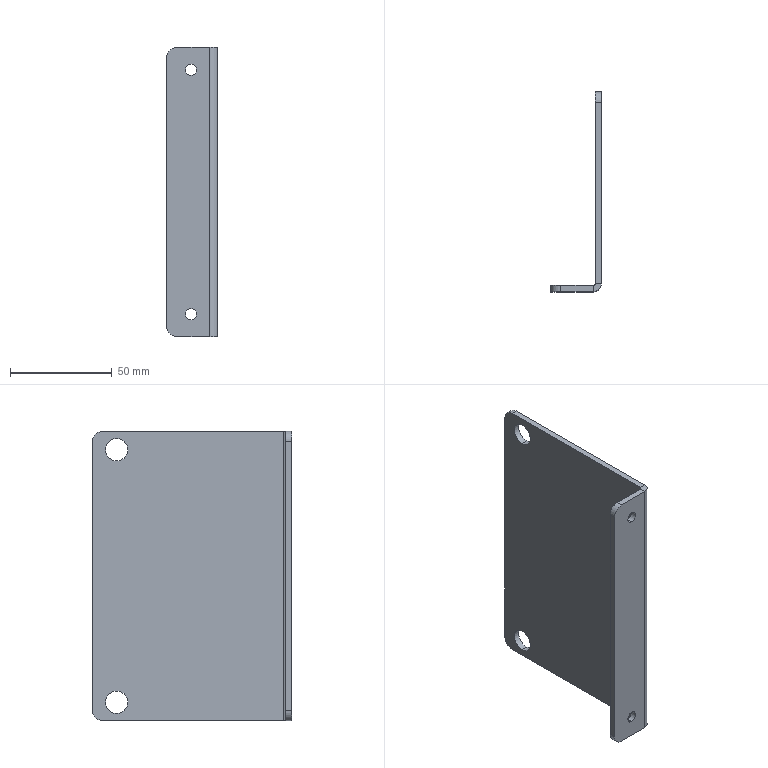Part | SolidWorks | features HoleWzd 2, BreakCorner 1, FlatPattern 1, SMBaseFlange 1, SheetMetal 1 | 1 solid | 26 faces | box 25 x 98 x 142 mm | volume 49886 mm3 | cylinder 14 | plane 12 | commonest cylinder face diameters 5.5 x4 10 x4 11 x4 2 x1 8 x1
STEP:
#1=CARTESIAN_POINT('',(12.,-3.,-62.75));
#2=VERTEX_POINT('',#1);
#3=CARTESIAN_POINT('',(12.,-3.,-57.25));
#4=VERTEX_POINT('',#3);
#5=CARTESIAN_POINT('',(12.,-3.,-60.));
#6=DIRECTION('',(0.,1.,0.));
#7=DIRECTION('',(0.,0.,1.));
#8=AXIS2_PLACEMENT_3D('',#5,#6,#7);
#9=CIRCLE('',#8,2.75);
#10=EDGE_CURVE('',#2,#4,#9,.T.);
#11=ORIENTED_EDGE('',*,*,#10,.F.);
#12=CARTESIAN_POINT('',(12.,0.,-62.75));
#13=VERTEX_POINT('',#12);
#14=CARTESIAN_POINT('',(12.,0.,-62.75));
#15=DIRECTION('',(0.,1.,0.));
#16=VECTOR('',#15,1000.);
#17=LINE('',#14,#16);
#18=EDGE_CURVE('',#2,#13,#17,.T.);
#19=ORIENTED_EDGE('',*,*,#18,.T.);
#20=CARTESIAN_POINT('',(12.,0.,-57.25));
#21=VERTEX_POINT('',#20);
#22=CARTESIAN_POINT('',(12.,0.,-60.));
#23=DIRECTION('',(0.,1.,0.));
#24=DIRECTION('',(0.,0.,1.));
#25=AXIS2_PLACEMENT_3D('',#22,#23,#24);
#26=CIRCLE('',#25,2.75);
#27=EDGE_CURVE('',#13,#21,#26,.T.);
#28=ORIENTED_EDGE('',*,*,#27,.T.);
#29=CARTESIAN_POINT('',(12.,0.,-57.25));
#30=DIRECTION('',(0.,1.,0.));
#31=VECTOR('',#30,1000.);
#32=LINE('',#29,#31);
#33=EDGE_CURVE('',#4,#21,#32,.T.);
#34=ORIENTED_EDGE('',*,*,#33,.F.);
#35=EDGE_LOOP('',(#11,#19,#28,#34));
#36=FACE_OUTER_BOUND('',#35,.T.);
#37=CARTESIAN_POINT('',(12.,0.,-60.));
#38=DIRECTION('',(0.,1.,0.));
#39=DIRECTION('',(0.,0.,1.));
#40=AXIS2_PLACEMENT_3D('',#37,#38,#39);
#41=CYLINDRICAL_SURFACE('',#40,2.75);
#42=ADVANCED_FACE('',(#36),#41,.F.);
#43=CARTESIAN_POINT('',(12.,-3.,57.25));
#44=VERTEX_POINT('',#43);
#45=CARTESIAN_POINT('',(12.,-3.,62.75));
#46=VERTEX_POINT('',#45);
#47=CARTESIAN_POINT('',(12.,-3.,60.));
#48=DIRECTION('',(0.,1.,0.));
#49=DIRECTION('',(0.,0.,1.));
#50=AXIS2_PLACEMENT_3D('',#47,#48,#49);
#51=CIRCLE('',#50,2.75);
#52=EDGE_CURVE('',#44,#46,#51,.T.);
#53=ORIENTED_EDGE('',*,*,#52,.F.);
#54=CARTESIAN_POINT('',(12.,0.,57.25));
#55=VERTEX_POINT('',#54);
#56=CARTESIAN_POINT('',(12.,0.,57.25));
#57=DIRECTION('',(0.,1.,0.));
#58=VECTOR('',#57,1000.);
#59=LINE('',#56,#58);
#60=EDGE_CURVE('',#44,#55,#59,.T.);
#61=ORIENTED_EDGE('',*,*,#60,.T.);
#62=CARTESIAN_POINT('',(12.,0.,62.75));
#63=VERTEX_POINT('',#62);
#64=CARTESIAN_POINT('',(12.,0.,60.));
#65=DIRECTION('',(0.,1.,0.));
#66=DIRECTION('',(0.,0.,1.));
#67=AXIS2_PLACEMENT_3D('',#64,#65,#66);
#68=CIRCLE('',#67,2.75);
#69=EDGE_CURVE('',#55,#63,#68,.T.);
#70=ORIENTED_EDGE('',*,*,#69,.T.);
#71=CARTESIAN_POINT('',(12.,0.,62.75));
#72=DIRECTION('',(0.,1.,0.));
#73=VECTOR('',#72,1000.);
#74=LINE('',#71,#73);
#75=EDGE_CURVE('',#46,#63,#74,.T.);
#76=ORIENTED_EDGE('',*,*,#75,.F.);
#77=EDGE_LOOP('',(#53,#61,#70,#76));
#78=FACE_OUTER_BOUND('',#77,.T.);
#79=CARTESIAN_POINT('',(12.,0.,60.));
#80=DIRECTION('',(0.,1.,0.));
#81=DIRECTION('',(0.,0.,1.));
#82=AXIS2_PLACEMENT_3D('',#79,#80,#81);
#83=CYLINDRICAL_SURFACE('',#82,2.75);
#84=ADVANCED_FACE('',(#78),#83,.F.);
#85=CARTESIAN_POINT('',(22.,83.,56.5));
#86=VERTEX_POINT('',#85);
#87=CARTESIAN_POINT('',(22.,83.,67.5));
#88=VERTEX_POINT('',#87);
#89=CARTESIAN_POINT('',(22.,83.,62.));
#90=DIRECTION('',(-1.,0.,0.));
#91=DIRECTION('',(0.,0.,1.));
#92=AXIS2_PLACEMENT_3D('',#89,#90,#91);
#93=CIRCLE('',#92,5.5);
#94=EDGE_CURVE('',#86,#88,#93,.T.);
#95=ORIENTED_EDGE('',*,*,#94,.T.);
#96=CARTESIAN_POINT('',(25.,83.,67.5));
#97=VERTEX_POINT('',#96);
#98=CARTESIAN_POINT('',(25.,83.,67.5));
#99=DIRECTION('',(1.,0.,0.));
#100=VECTOR('',#99,1000.);
#101=LINE('',#98,#100);
#102=EDGE_CURVE('',#88,#97,#101,.T.);
#103=ORIENTED_EDGE('',*,*,#102,.T.);
#104=CARTESIAN_POINT('',(25.,83.,56.5));
#105=VERTEX_POINT('',#104);
#106=CARTESIAN_POINT('',(25.,83.,62.));
#107=DIRECTION('',(1.,0.,0.));
#108=DIRECTION('',(0.,0.,-1.));
#109=AXIS2_PLACEMENT_3D('',#106,#107,#108);
#110=CIRCLE('',#109,5.5);
#111=EDGE_CURVE('',#97,#105,#110,.T.);
#112=ORIENTED_EDGE('',*,*,#111,.T.);
#113=CARTESIAN_POINT('',(25.,83.,56.5));
#114=DIRECTION('',(1.,0.,0.));
#115=VECTOR('',#114,1000.);
#116=LINE('',#113,#115);
#117=EDGE_CURVE('',#86,#105,#116,.T.);
#118=ORIENTED_EDGE('',*,*,#117,.F.);
#119=EDGE_LOOP('',(#95,#103,#112,#118));
#120=FACE_OUTER_BOUND('',#119,.T.);
#121=CARTESIAN_POINT('',(25.,83.,62.));
#122=DIRECTION('',(1.,0.,0.));
#123=DIRECTION('',(0.,0.,-1.));
#124=AXIS2_PLACEMENT_3D('',#121,#122,#123);
#125=CYLINDRICAL_SURFACE('',#124,5.5);
#126=ADVANCED_FACE('',(#120),#125,.F.);
#127=CARTESIAN_POINT('',(22.,83.,-67.5));
#128=VERTEX_POINT('',#127);
#129=CARTESIAN_POINT('',(22.,83.,-56.5));
#130=VERTEX_POINT('',#129);
#131=CARTESIAN_POINT('',(22.,83.,-62.));
#132=DIRECTION('',(-1.,0.,0.));
#133=DIRECTION('',(0.,0.,1.));
#134=AXIS2_PLACEMENT_3D('',#131,#132,#133);
#135=CIRCLE('',#134,5.5);
#136=EDGE_CURVE('',#128,#130,#135,.T.);
#137=ORIENTED_EDGE('',*,*,#136,.T.);
#138=CARTESIAN_POINT('',(25.,83.,-56.5));
#139=VERTEX_POINT('',#138);
#140=CARTESIAN_POINT('',(25.,83.,-56.5));
#141=DIRECTION('',(1.,0.,0.));
#142=VECTOR('',#141,1000.);
#143=LINE('',#140,#142);
#144=EDGE_CURVE('',#130,#139,#143,.T.);
#145=ORIENTED_EDGE('',*,*,#144,.T.);
#146=CARTESIAN_POINT('',(25.,83.,-67.5));
#147=VERTEX_POINT('',#146);
#148=CARTESIAN_POINT('',(25.,83.,-62.));
#149=DIRECTION('',(1.,0.,0.));
#150=DIRECTION('',(0.,0.,-1.));
#151=AXIS2_PLACEMENT_3D('',#148,#149,#150);
#152=CIRCLE('',#151,5.5);
#153=EDGE_CURVE('',#139,#147,#152,.T.);
#154=ORIENTED_EDGE('',*,*,#153,.T.);
#155=CARTESIAN_POINT('',(25.,83.,-67.5));
#156=DIRECTION('',(1.,0.,0.));
#157=VECTOR('',#156,1000.);
#158=LINE('',#155,#157);
#159=EDGE_CURVE('',#128,#147,#158,.T.);
#160=ORIENTED_EDGE('',*,*,#159,.F.);
#161=EDGE_LOOP('',(#137,#145,#154,#160));
#162=FACE_OUTER_BOUND('',#161,.T.);
#163=CARTESIAN_POINT('',(25.,83.,-62.));
#164=DIRECTION('',(1.,0.,0.));
#165=DIRECTION('',(0.,0.,-1.));
#166=AXIS2_PLACEMENT_3D('',#163,#164,#165);
#167=CYLINDRICAL_SURFACE('',#166,5.5);
#168=ADVANCED_FACE('',(#162),#167,.F.);
#169=CARTESIAN_POINT('',(22.,1.,71.));
#170=VERTEX_POINT('',#169);
#171=CARTESIAN_POINT('',(25.,1.,71.));
#172=VERTEX_POINT('',#171);
#173=CARTESIAN_POINT('',(22.,1.,71.));
#174=DIRECTION('',(1.,0.,0.));
#175=VECTOR('',#174,1000.);
#176=LINE('',#173,#175);
#177=EDGE_CURVE('',#170,#172,#176,.T.);
#178=ORIENTED_EDGE('',*,*,#177,.F.);
#179=CARTESIAN_POINT('',(21.,0.,71.));
#180=VERTEX_POINT('',#179);
#181=CARTESIAN_POINT('',(21.,1.,71.));
#182=DIRECTION('',(0.,0.,1.));
#183=DIRECTION('',(-1.,0.,0.));
#184=AXIS2_PLACEMENT_3D('',#181,#182,#183);
#185=CIRCLE('',#184,1.);
#186=EDGE_CURVE('',#180,#170,#185,.T.);
#187=ORIENTED_EDGE('',*,*,#186,.F.);
#188=CARTESIAN_POINT('',(21.,-3.,71.));
#189=VERTEX_POINT('',#188);
#190=CARTESIAN_POINT('',(21.,-3.,71.));
#191=DIRECTION('',(0.,1.,0.));
#192=VECTOR('',#191,1000.);
#193=LINE('',#190,#192);
#194=EDGE_CURVE('',#189,#180,#193,.T.);
#195=ORIENTED_EDGE('',*,*,#194,.F.);
#196=CARTESIAN_POINT('',(21.,1.,71.));
#197=DIRECTION('',(0.,0.,1.));
#198=DIRECTION('',(1.,0.,0.));
#199=AXIS2_PLACEMENT_3D('',#196,#197,#198);
#200=CIRCLE('',#199,4.);
#201=EDGE_CURVE('',#189,#172,#200,.T.);
#202=ORIENTED_EDGE('',*,*,#201,.T.);
#203=EDGE_LOOP('',(#178,#187,#195,#202));
#204=FACE_OUTER_BOUND('',#203,.T.);
#205=CARTESIAN_POINT('',(22.,1.,71.));
#206=DIRECTION('',(0.,0.,1.));
#207=DIRECTION('',(1.,0.,0.));
#208=AXIS2_PLACEMENT_3D('',#205,#206,#207);
#209=PLANE('',#208);
#210=ADVANCED_FACE('',(#204),#209,.T.);
#211=CARTESIAN_POINT('',(25.,90.,71.));
#212=VERTEX_POINT('',#211);
#213=CARTESIAN_POINT('',(25.,0.,71.));
#214=DIRECTION('',(0.,1.,0.));
#215=VECTOR('',#214,1000.);
#216=LINE('',#213,#215);
#217=EDGE_CURVE('',#172,#212,#216,.T.);
#218=ORIENTED_EDGE('',*,*,#217,.T.);
#219=CARTESIAN_POINT('',(22.,90.,71.));
#220=VERTEX_POINT('',#219);
#221=CARTESIAN_POINT('',(21.,90.,71.));
#222=DIRECTION('',(-1.,0.,0.));
#223=VECTOR('',#222,1000.);
#224=LINE('',#221,#223);
#225=EDGE_CURVE('',#212,#220,#224,.T.);
#226=ORIENTED_EDGE('',*,*,#225,.T.);
#227=CARTESIAN_POINT('',(22.,0.,71.));
#228=DIRECTION('',(0.,1.,0.));
#229=VECTOR('',#228,1000.);
#230=LINE('',#227,#229);
#231=EDGE_CURVE('',#170,#220,#230,.T.);
#232=ORIENTED_EDGE('',*,*,#231,.F.);
#233=ORIENTED_EDGE('',*,*,#177,.T.);
#234=EDGE_LOOP('',(#218,#226,#232,#233));
#235=FACE_OUTER_BOUND('',#234,.T.);
#236=CARTESIAN_POINT('',(21.,-3.,71.));
#237=DIRECTION('',(0.,0.,1.));
#238=DIRECTION('',(1.,0.,0.));
#239=AXIS2_PLACEMENT_3D('',#236,#237,#238);
#240=PLANE('',#239);
#241=ADVANCED_FACE('',(#235),#240,.T.);
#242=CARTESIAN_POINT('',(21.,0.,-71.));
#243=VERTEX_POINT('',#242);
#244=CARTESIAN_POINT('',(21.,-3.,-71.));
#245=VERTEX_POINT('',#244);
#246=CARTESIAN_POINT('',(21.,0.,-71.));
#247=DIRECTION('',(0.,-1.,0.));
#248=VECTOR('',#247,1000.);
#249=LINE('',#246,#248);
#250=EDGE_CURVE('',#243,#245,#249,.T.);
#251=ORIENTED_EDGE('',*,*,#250,.F.);
#252=CARTESIAN_POINT('',(22.,1.,-71.));
#253=VERTEX_POINT('',#252);
#254=CARTESIAN_POINT('',(21.,1.,-71.));
#255=DIRECTION('',(0.,0.,1.));
#256=DIRECTION('',(-1.,0.,0.));
#257=AXIS2_PLACEMENT_3D('',#254,#255,#256);
#258=CIRCLE('',#257,1.);
#259=EDGE_CURVE('',#243,#253,#258,.T.);
#260=ORIENTED_EDGE('',*,*,#259,.T.);
#261=CARTESIAN_POINT('',(25.,1.,-71.));
#262=VERTEX_POINT('',#261);
#263=CARTESIAN_POINT('',(25.,1.,-71.));
#264=DIRECTION('',(-1.,0.,0.));
#265=VECTOR('',#264,1000.);
#266=LINE('',#263,#265);
#267=EDGE_CURVE('',#262,#253,#266,.T.);
#268=ORIENTED_EDGE('',*,*,#267,.F.);
#269=CARTESIAN_POINT('',(21.,1.,-71.));
#270=DIRECTION('',(0.,0.,1.));
#271=DIRECTION('',(1.,0.,0.));
#272=AXIS2_PLACEMENT_3D('',#269,#270,#271);
#273=CIRCLE('',#272,4.);
#274=EDGE_CURVE('',#245,#262,#273,.T.);
#275=ORIENTED_EDGE('',*,*,#274,.F.);
#276=EDGE_LOOP('',(#251,#260,#268,#275));
#277=FACE_OUTER_BOUND('',#276,.T.);
#278=CARTESIAN_POINT('',(21.,0.,-71.));
#279=DIRECTION('',(0.,0.,-1.));
#280=DIRECTION('',(-1.,0.,0.));
#281=AXIS2_PLACEMENT_3D('',#278,#279,#280);
#282=PLANE('',#281);
#283=ADVANCED_FACE('',(#277),#282,.T.);
#284=CARTESIAN_POINT('',(5.,-3.,-71.));
#285=VERTEX_POINT('',#284);
#286=CARTESIAN_POINT('',(0.,-3.,-71.));
#287=DIRECTION('',(1.,0.,0.));
#288=VECTOR('',#287,1000.);
#289=LINE('',#286,#288);
#290=EDGE_CURVE('',#285,#245,#289,.T.);
#291=ORIENTED_EDGE('',*,*,#290,.F.);
#292=CARTESIAN_POINT('',(5.,0.,-71.));
#293=VERTEX_POINT('',#292);
#294=CARTESIAN_POINT('',(5.,1.,-71.));
#295=DIRECTION('',(0.,1.,0.));
#296=VECTOR('',#295,1000.);
#297=LINE('',#294,#296);
#298=EDGE_CURVE('',#285,#293,#297,.T.);
#299=ORIENTED_EDGE('',*,*,#298,.T.);
#300=CARTESIAN_POINT('',(0.,0.,-71.));
#301=DIRECTION('',(1.,0.,0.));
#302=VECTOR('',#301,1000.);
#303=LINE('',#300,#302);
#304=EDGE_CURVE('',#293,#243,#303,.T.);
#305=ORIENTED_EDGE('',*,*,#304,.T.);
#306=ORIENTED_EDGE('',*,*,#250,.T.);
#307=EDGE_LOOP('',(#291,#299,#305,#306));
#308=FACE_OUTER_BOUND('',#307,.T.);
#309=CARTESIAN_POINT('',(25.,1.,-71.));
#310=DIRECTION('',(0.,0.,-1.));
#311=DIRECTION('',(-1.,0.,0.));
#312=AXIS2_PLACEMENT_3D('',#309,#310,#311);
#313=PLANE('',#312);
#314=ADVANCED_FACE('',(#308),#313,.T.);
#315=CARTESIAN_POINT('',(25.,83.,62.));
#316=DIRECTION('',(1.,0.,0.));
#317=DIRECTION('',(0.,0.,-1.));
#318=AXIS2_PLACEMENT_3D('',#315,#316,#317);
#319=CIRCLE('',#318,5.5);
#320=EDGE_CURVE('',#105,#97,#319,.T.);
#321=ORIENTED_EDGE('',*,*,#320,.F.);
#322=ORIENTED_EDGE('',*,*,#111,.F.);
#323=EDGE_LOOP('',(#321,#322));
#324=FACE_BOUND('',#323,.T.);
#325=CARTESIAN_POINT('',(25.,83.,-62.));
#326=DIRECTION('',(1.,0.,0.));
#327=DIRECTION('',(0.,0.,-1.));
#328=AXIS2_PLACEMENT_3D('',#325,#326,#327);
#329=CIRCLE('',#328,5.5);
#330=EDGE_CURVE('',#147,#139,#329,.T.);
#331=ORIENTED_EDGE('',*,*,#330,.F.);
#332=ORIENTED_EDGE('',*,*,#153,.F.);
#333=EDGE_LOOP('',(#331,#332));
#334=FACE_BOUND('',#333,.T.);
#335=CARTESIAN_POINT('',(25.,95.,66.));
#336=VERTEX_POINT('',#335);
#337=CARTESIAN_POINT('',(25.,95.,-66.));
#338=VERTEX_POINT('',#337);
#339=CARTESIAN_POINT('',(25.,95.,71.));
#340=DIRECTION('',(0.,0.,-1.));
#341=VECTOR('',#340,1000.);
#342=LINE('',#339,#341);
#343=EDGE_CURVE('',#336,#338,#342,.T.);
#344=ORIENTED_EDGE('',*,*,#343,.F.);
#345=CARTESIAN_POINT('',(25.,90.,66.));
#346=DIRECTION('',(1.,0.,0.));
#347=DIRECTION('',(0.,0.,1.));
#348=AXIS2_PLACEMENT_3D('',#345,#346,#347);
#349=CIRCLE('',#348,5.);
#350=EDGE_CURVE('',#336,#212,#349,.T.);
#351=ORIENTED_EDGE('',*,*,#350,.T.);
#352=ORIENTED_EDGE('',*,*,#217,.F.);
#353=CARTESIAN_POINT('',(25.,1.,71.));
#354=DIRECTION('',(0.,0.,-1.));
#355=VECTOR('',#354,1000.);
#356=LINE('',#353,#355);
#357=EDGE_CURVE('',#172,#262,#356,.T.);
#358=ORIENTED_EDGE('',*,*,#357,.T.);
#359=CARTESIAN_POINT('',(25.,90.,-71.));
#360=VERTEX_POINT('',#359);
#361=CARTESIAN_POINT('',(25.,0.,-71.));
#362=DIRECTION('',(0.,1.,0.));
#363=VECTOR('',#362,1000.);
#364=LINE('',#361,#363);
#365=EDGE_CURVE('',#262,#360,#364,.T.);
#366=ORIENTED_EDGE('',*,*,#365,.T.);
#367=CARTESIAN_POINT('',(25.,90.,-66.));
#368=DIRECTION('',(1.,0.,0.));
#369=DIRECTION('',(0.,0.,1.));
#370=AXIS2_PLACEMENT_3D('',#367,#368,#369);
#371=CIRCLE('',#370,5.);
#372=EDGE_CURVE('',#360,#338,#371,.T.);
#373=ORIENTED_EDGE('',*,*,#372,.T.);
#374=EDGE_LOOP('',(#344,#351,#352,#358,#366,#373));
#375=FACE_OUTER_BOUND('',#374,.T.);
#376=CARTESIAN_POINT('',(25.,0.,71.));
#377=DIRECTION('',(-1.,0.,0.));
#378=DIRECTION('',(0.,0.,1.));
#379=AXIS2_PLACEMENT_3D('',#376,#377,#378);
#380=PLANE('',#379);
#381=ADVANCED_FACE('',(#324,#334,#375),#380,.F.);
#382=CARTESIAN_POINT('',(22.,95.,66.));
#383=VERTEX_POINT('',#382);
#384=CARTESIAN_POINT('',(22.,95.,-66.));
#385=VERTEX_POINT('',#384);
#386=CARTESIAN_POINT('',(22.,95.,71.));
#387=DIRECTION('',(0.,0.,-1.));
#388=VECTOR('',#387,1000.);
#389=LINE('',#386,#388);
#390=EDGE_CURVE('',#383,#385,#389,.T.);
#391=ORIENTED_EDGE('',*,*,#390,.F.);
#392=CARTESIAN_POINT('',(22.,95.,66.));
#393=DIRECTION('',(1.,0.,0.));
#394=VECTOR('',#393,1000.);
#395=LINE('',#392,#394);
#396=EDGE_CURVE('',#383,#336,#395,.T.);
#397=ORIENTED_EDGE('',*,*,#396,.T.);
#398=ORIENTED_EDGE('',*,*,#343,.T.);
#399=CARTESIAN_POINT('',(22.,95.,-66.));
#400=DIRECTION('',(-1.,0.,0.));
#401=VECTOR('',#400,1000.);
#402=LINE('',#399,#401);
#403=EDGE_CURVE('',#338,#385,#402,.T.);
#404=ORIENTED_EDGE('',*,*,#403,.T.);
#405=EDGE_LOOP('',(#391,#397,#398,#404));
#406=FACE_OUTER_BOUND('',#405,.T.);
#407=CARTESIAN_POINT('',(22.,95.,71.));
#408=DIRECTION('',(0.,1.,0.));
#409=DIRECTION('',(0.,0.,1.));
#410=AXIS2_PLACEMENT_3D('',#407,#408,#409);
#411=PLANE('',#410);
#412=ADVANCED_FACE('',(#406),#411,.T.);
#413=ORIENTED_EDGE('',*,*,#94,.F.);
#414=CARTESIAN_POINT('',(22.,83.,62.));
#415=DIRECTION('',(-1.,0.,0.));
#416=DIRECTION('',(0.,0.,1.));
#417=AXIS2_PLACEMENT_3D('',#414,#415,#416);
#418=CIRCLE('',#417,5.5);
#419=EDGE_CURVE('',#88,#86,#418,.T.);
#420=ORIENTED_EDGE('',*,*,#419,.F.);
#421=EDGE_LOOP('',(#413,#420));
#422=FACE_BOUND('',#421,.T.);
#423=ORIENTED_EDGE('',*,*,#136,.F.);
#424=CARTESIAN_POINT('',(22.,83.,-62.));
#425=DIRECTION('',(-1.,0.,0.));
#426=DIRECTION('',(0.,0.,1.));
#427=AXIS2_PLACEMENT_3D('',#424,#425,#426);
#428=CIRCLE('',#427,5.5);
#429=EDGE_CURVE('',#130,#128,#428,.T.);
#430=ORIENTED_EDGE('',*,*,#429,.F.);
#431=EDGE_LOOP('',(#423,#430));
#432=FACE_BOUND('',#431,.T.);
#433=ORIENTED_EDGE('',*,*,#231,.T.);
#434=CARTESIAN_POINT('',(22.,90.,66.));
#435=DIRECTION('',(-1.,0.,0.));
#436=DIRECTION('',(0.,0.,1.));
#437=AXIS2_PLACEMENT_3D('',#434,#435,#436);
#438=CIRCLE('',#437,5.);
#439=EDGE_CURVE('',#220,#383,#438,.T.);
#440=ORIENTED_EDGE('',*,*,#439,.T.);
#441=ORIENTED_EDGE('',*,*,#390,.T.);
#442=CARTESIAN_POINT('',(22.,90.,-71.));
#443=VERTEX_POINT('',#442);
#444=CARTESIAN_POINT('',(22.,90.,-66.));
#445=DIRECTION('',(-1.,0.,0.));
#446=DIRECTION('',(0.,0.,1.));
#447=AXIS2_PLACEMENT_3D('',#444,#445,#446);
#448=CIRCLE('',#447,5.);
#449=EDGE_CURVE('',#385,#443,#448,.T.);
#450=ORIENTED_EDGE('',*,*,#449,.T.);
#451=CARTESIAN_POINT('',(22.,0.,-71.));
#452=DIRECTION('',(0.,1.,0.));
#453=VECTOR('',#452,1000.);
#454=LINE('',#451,#453);
#455=EDGE_CURVE('',#253,#443,#454,.T.);
#456=ORIENTED_EDGE('',*,*,#455,.F.);
#457=CARTESIAN_POINT('',(22.,1.,71.));
#458=DIRECTION('',(0.,0.,-1.));
#459=VECTOR('',#458,1000.);
#460=LINE('',#457,#459);
#461=EDGE_CURVE('',#170,#253,#460,.T.);
#462=ORIENTED_EDGE('',*,*,#461,.F.);
#463=EDGE_LOOP('',(#433,#440,#441,#450,#456,#462));
#464=FACE_OUTER_BOUND('',#463,.T.);
#465=CARTESIAN_POINT('',(22.,0.,71.));
#466=DIRECTION('',(-1.,0.,0.));
#467=DIRECTION('',(0.,0.,1.));
#468=AXIS2_PLACEMENT_3D('',#465,#466,#467);
#469=PLANE('',#468);
#470=ADVANCED_FACE('',(#422,#432,#464),#469,.T.);
#471=ORIENTED_EDGE('',*,*,#259,.F.);
#472=CARTESIAN_POINT('',(21.,0.,71.));
#473=DIRECTION('',(0.,0.,-1.));
#474=VECTOR('',#473,1000.);
#475=LINE('',#472,#474);
#476=EDGE_CURVE('',#180,#243,#475,.T.);
#477=ORIENTED_EDGE('',*,*,#476,.F.);
#478=ORIENTED_EDGE('',*,*,#186,.T.);
#479=ORIENTED_EDGE('',*,*,#461,.T.);
#480=EDGE_LOOP('',(#471,#477,#478,#479));
#481=FACE_OUTER_BOUND('',#480,.T.);
#482=CARTESIAN_POINT('',(21.,1.,71.));
#483=DIRECTION('',(0.,0.,-1.));
#484=DIRECTION('',(-1.,0.,0.));
#485=AXIS2_PLACEMENT_3D('',#482,#483,#484);
#486=CYLINDRICAL_SURFACE('',#485,1.);
#487=ADVANCED_FACE('',(#481),#486,.F.);
#488=CARTESIAN_POINT('',(12.,0.,-60.));
#489=DIRECTION('',(0.,1.,0.));
#490=DIRECTION('',(0.,0.,1.));
#491=AXIS2_PLACEMENT_3D('',#488,#489,#490);
#492=CIRCLE('',#491,2.75);
#493=EDGE_CURVE('',#21,#13,#492,.T.);
#494=ORIENTED_EDGE('',*,*,#493,.F.);
#495=ORIENTED_EDGE('',*,*,#27,.F.);
#496=EDGE_LOOP('',(#494,#495));
#497=FACE_BOUND('',#496,.T.);
#498=CARTESIAN_POINT('',(12.,0.,60.));
#499=DIRECTION('',(0.,1.,0.));
#500=DIRECTION('',(0.,0.,1.));
#501=AXIS2_PLACEMENT_3D('',#498,#499,#500);
#502=CIRCLE('',#501,2.75);
#503=EDGE_CURVE('',#63,#55,#502,.T.);
#504=ORIENTED_EDGE('',*,*,#503,.F.);
#505=ORIENTED_EDGE('',*,*,#69,.F.);
#506=EDGE_LOOP('',(#504,#505));
#507=FACE_BOUND('',#506,.T.);
#508=CARTESIAN_POINT('',(0.,0.,66.));
#509=VERTEX_POINT('',#508);
#510=CARTESIAN_POINT('',(0.,0.,-66.));
#511=VERTEX_POINT('',#510);
#512=CARTESIAN_POINT('',(0.,0.,71.));
#513=DIRECTION('',(0.,0.,-1.));
#514=VECTOR('',#513,1000.);
#515=LINE('',#512,#514);
#516=EDGE_CURVE('',#509,#511,#515,.T.);
#517=ORIENTED_EDGE('',*,*,#516,.F.);
#518=CARTESIAN_POINT('',(5.,0.,71.));
#519=VERTEX_POINT('',#518);
#520=CARTESIAN_POINT('',(5.,0.,66.));
#521=DIRECTION('',(0.,1.,0.));
#522=DIRECTION('',(0.,0.,1.));
#523=AXIS2_PLACEMENT_3D('',#520,#521,#522);
#524=CIRCLE('',#523,5.);
#525=EDGE_CURVE('',#509,#519,#524,.T.);
#526=ORIENTED_EDGE('',*,*,#525,.T.);
#527=CARTESIAN_POINT('',(0.,0.,71.));
#528=DIRECTION('',(1.,0.,0.));
#529=VECTOR('',#528,1000.);
#530=LINE('',#527,#529);
#531=EDGE_CURVE('',#519,#180,#530,.T.);
#532=ORIENTED_EDGE('',*,*,#531,.T.);
#533=ORIENTED_EDGE('',*,*,#476,.T.);
#534=ORIENTED_EDGE('',*,*,#304,.F.);
#535=CARTESIAN_POINT('',(5.,0.,-66.));
#536=DIRECTION('',(0.,1.,0.));
#537=DIRECTION('',(0.,0.,1.));
#538=AXIS2_PLACEMENT_3D('',#535,#536,#537);
#539=CIRCLE('',#538,5.);
#540=EDGE_CURVE('',#293,#511,#539,.T.);
#541=ORIENTED_EDGE('',*,*,#540,.T.);
#542=EDGE_LOOP('',(#517,#526,#532,#533,#534,#541));
#543=FACE_OUTER_BOUND('',#542,.T.);
#544=CARTESIAN_POINT('',(0.,0.,71.));
#545=DIRECTION('',(0.,1.,0.));
#546=DIRECTION('',(0.,0.,1.));
#547=AXIS2_PLACEMENT_3D('',#544,#545,#546);
#548=PLANE('',#547);
#549=ADVANCED_FACE('',(#497,#507,#543),#548,.T.);
#550=CARTESIAN_POINT('',(0.,-3.,66.));
#551=VERTEX_POINT('',#550);
#552=CARTESIAN_POINT('',(0.,-3.,-66.));
#553=VERTEX_POINT('',#552);
#554=CARTESIAN_POINT('',(0.,-3.,71.));
#555=DIRECTION('',(0.,0.,-1.));
#556=VECTOR('',#555,1000.);
#557=LINE('',#554,#556);
#558=EDGE_CURVE('',#551,#553,#557,.T.);
#559=ORIENTED_EDGE('',*,*,#558,.F.);
#560=CARTESIAN_POINT('',(0.,0.,66.));
#561=DIRECTION('',(0.,1.,0.));
#562=VECTOR('',#561,1000.);
#563=LINE('',#560,#562);
#564=EDGE_CURVE('',#551,#509,#563,.T.);
#565=ORIENTED_EDGE('',*,*,#564,.T.);
#566=ORIENTED_EDGE('',*,*,#516,.T.);
#567=CARTESIAN_POINT('',(0.,-3.,-66.));
#568=DIRECTION('',(0.,-1.,0.));
#569=VECTOR('',#568,1000.);
#570=LINE('',#567,#569);
#571=EDGE_CURVE('',#511,#553,#570,.T.);
#572=ORIENTED_EDGE('',*,*,#571,.T.);
#573=EDGE_LOOP('',(#559,#565,#566,#572));
#574=FACE_OUTER_BOUND('',#573,.T.);
#575=CARTESIAN_POINT('',(0.,-3.,71.));
#576=DIRECTION('',(-1.,0.,0.));
#577=DIRECTION('',(0.,0.,1.));
#578=AXIS2_PLACEMENT_3D('',#575,#576,#577);
#579=PLANE('',#578);
#580=ADVANCED_FACE('',(#574),#579,.T.);
#581=CARTESIAN_POINT('',(12.,-3.,-60.));
#582=DIRECTION('',(0.,1.,0.));
#583=DIRECTION('',(0.,0.,1.));
#584=AXIS2_PLACEMENT_3D('',#581,#582,#583);
#585=CIRCLE('',#584,2.75);
#586=EDGE_CURVE('',#4,#2,#585,.T.);
#587=ORIENTED_EDGE('',*,*,#586,.T.);
#588=ORIENTED_EDGE('',*,*,#10,.T.);
#589=EDGE_LOOP('',(#587,#588));
#590=FACE_BOUND('',#589,.T.);
#591=CARTESIAN_POINT('',(12.,-3.,60.));
#592=DIRECTION('',(0.,1.,0.));
#593=DIRECTION('',(0.,0.,1.));
#594=AXIS2_PLACEMENT_3D('',#591,#592,#593);
#595=CIRCLE('',#594,2.75);
#596=EDGE_CURVE('',#46,#44,#595,.T.);
#597=ORIENTED_EDGE('',*,*,#596,.T.);
#598=ORIENTED_EDGE('',*,*,#52,.T.);
#599=EDGE_LOOP('',(#597,#598));
#600=FACE_BOUND('',#599,.T.);
#601=CARTESIAN_POINT('',(5.,-3.,71.));
#602=VERTEX_POINT('',#601);
#603=CARTESIAN_POINT('',(0.,-3.,71.));
#604=DIRECTION('',(1.,0.,0.));
#605=VECTOR('',#604,1000.);
#606=LINE('',#603,#605);
#607=EDGE_CURVE('',#602,#189,#606,.T.);
#608=ORIENTED_EDGE('',*,*,#607,.F.);
#609=CARTESIAN_POINT('',(5.,-3.,66.));
#610=DIRECTION('',(0.,-1.,0.));
#611=DIRECTION('',(0.,0.,1.));
#612=AXIS2_PLACEMENT_3D('',#609,#610,#611);
#613=CIRCLE('',#612,5.);
#614=EDGE_CURVE('',#602,#551,#613,.T.);
#615=ORIENTED_EDGE('',*,*,#614,.T.);
#616=ORIENTED_EDGE('',*,*,#558,.T.);
#617=CARTESIAN_POINT('',(5.,-3.,-66.));
#618=DIRECTION('',(0.,-1.,0.));
#619=DIRECTION('',(0.,0.,1.));
#620=AXIS2_PLACEMENT_3D('',#617,#618,#619);
#621=CIRCLE('',#620,5.);
#622=EDGE_CURVE('',#553,#285,#621,.T.);
#623=ORIENTED_EDGE('',*,*,#622,.T.);
#624=ORIENTED_EDGE('',*,*,#290,.T.);
#625=CARTESIAN_POINT('',(21.,-3.,71.));
#626=DIRECTION('',(0.,0.,-1.));
#627=VECTOR('',#626,1000.);
#628=LINE('',#625,#627);
#629=EDGE_CURVE('',#189,#245,#628,.T.);
#630=ORIENTED_EDGE('',*,*,#629,.F.);
#631=EDGE_LOOP('',(#608,#615,#616,#623,#624,#630));
#632=FACE_OUTER_BOUND('',#631,.T.);
#633=CARTESIAN_POINT('',(0.,-3.,71.));
#634=DIRECTION('',(0.,1.,0.));
#635=DIRECTION('',(0.,0.,1.));
#636=AXIS2_PLACEMENT_3D('',#633,#634,#635);
#637=PLANE('',#636);
#638=ADVANCED_FACE('',(#590,#600,#632),#637,.F.);
#639=ORIENTED_EDGE('',*,*,#274,.T.);
#640=ORIENTED_EDGE('',*,*,#357,.F.);
#641=ORIENTED_EDGE('',*,*,#201,.F.);
#642=ORIENTED_EDGE('',*,*,#629,.T.);
#643=EDGE_LOOP('',(#639,#640,#641,#642));
#644=FACE_OUTER_BOUND('',#643,.T.);
#645=CARTESIAN_POINT('',(21.,1.,71.));
#646=DIRECTION('',(0.,0.,-1.));
#647=DIRECTION('',(-1.,0.,0.));
#648=AXIS2_PLACEMENT_3D('',#645,#646,#647);
#649=CYLINDRICAL_SURFACE('',#648,4.);
#650=ADVANCED_FACE('',(#644),#649,.T.);
#651=ORIENTED_EDGE('',*,*,#531,.F.);
#652=CARTESIAN_POINT('',(5.,-3.,71.));
#653=DIRECTION('',(0.,-1.,0.));
#654=VECTOR('',#653,1000.);
#655=LINE('',#652,#654);
#656=EDGE_CURVE('',#519,#602,#655,.T.);
#657=ORIENTED_EDGE('',*,*,#656,.T.);
#658=ORIENTED_EDGE('',*,*,#607,.T.);
#659=ORIENTED_EDGE('',*,*,#194,.T.);
#660=EDGE_LOOP('',(#651,#657,#658,#659));
#661=FACE_OUTER_BOUND('',#660,.T.);
#662=CARTESIAN_POINT('',(21.,1.,71.));
#663=DIRECTION('',(0.,0.,-1.));
#664=DIRECTION('',(-1.,0.,0.));
#665=AXIS2_PLACEMENT_3D('',#662,#663,#664);
#666=PLANE('',#665);
#667=ADVANCED_FACE('',(#661),#666,.F.);
#668=ORIENTED_EDGE('',*,*,#455,.T.);
#669=CARTESIAN_POINT('',(21.,90.,-71.));
#670=DIRECTION('',(1.,0.,0.));
#671=VECTOR('',#670,1000.);
#672=LINE('',#669,#671);
#673=EDGE_CURVE('',#443,#360,#672,.T.);
#674=ORIENTED_EDGE('',*,*,#673,.T.);
#675=ORIENTED_EDGE('',*,*,#365,.F.);
#676=ORIENTED_EDGE('',*,*,#267,.T.);
#677=EDGE_LOOP('',(#668,#674,#675,#676));
#678=FACE_OUTER_BOUND('',#677,.T.);
#679=CARTESIAN_POINT('',(21.,1.,-71.));
#680=DIRECTION('',(0.,0.,-1.));
#681=DIRECTION('',(-1.,0.,0.));
#682=AXIS2_PLACEMENT_3D('',#679,#680,#681);
#683=PLANE('',#682);
#684=ADVANCED_FACE('',(#678),#683,.T.);
#685=ORIENTED_EDGE('',*,*,#614,.F.);
#686=ORIENTED_EDGE('',*,*,#656,.F.);
#687=ORIENTED_EDGE('',*,*,#525,.F.);
#688=ORIENTED_EDGE('',*,*,#564,.F.);
#689=EDGE_LOOP('',(#685,#686,#687,#688));
#690=FACE_OUTER_BOUND('',#689,.T.);
#691=CARTESIAN_POINT('',(5.,-3.,66.));
#692=DIRECTION('',(0.,-1.,0.));
#693=DIRECTION('',(0.,0.,-1.));
#694=AXIS2_PLACEMENT_3D('',#691,#692,#693);
#695=CYLINDRICAL_SURFACE('',#694,5.);
#696=ADVANCED_FACE('',(#690),#695,.T.);
#697=ORIENTED_EDGE('',*,*,#622,.F.);
#698=ORIENTED_EDGE('',*,*,#571,.F.);
#699=ORIENTED_EDGE('',*,*,#540,.F.);
#700=ORIENTED_EDGE('',*,*,#298,.F.);
#701=EDGE_LOOP('',(#697,#698,#699,#700));
#702=FACE_OUTER_BOUND('',#701,.T.);
#703=CARTESIAN_POINT('',(5.,1.,-66.));
#704=DIRECTION('',(0.,1.,0.));
#705=DIRECTION('',(0.,0.,1.));
#706=AXIS2_PLACEMENT_3D('',#703,#704,#705);
#707=CYLINDRICAL_SURFACE('',#706,5.);
#708=ADVANCED_FACE('',(#702),#707,.T.);
#709=ORIENTED_EDGE('',*,*,#439,.F.);
#710=ORIENTED_EDGE('',*,*,#225,.F.);
#711=ORIENTED_EDGE('',*,*,#350,.F.);
#712=ORIENTED_EDGE('',*,*,#396,.F.);
#713=EDGE_LOOP('',(#709,#710,#711,#712));
#714=FACE_OUTER_BOUND('',#713,.T.);
#715=CARTESIAN_POINT('',(22.,90.,66.));
#716=DIRECTION('',(1.,0.,0.));
#717=DIRECTION('',(0.,0.,-1.));
#718=AXIS2_PLACEMENT_3D('',#715,#716,#717);
#719=CYLINDRICAL_SURFACE('',#718,5.);
#720=ADVANCED_FACE('',(#714),#719,.T.);
#721=ORIENTED_EDGE('',*,*,#449,.F.);
#722=ORIENTED_EDGE('',*,*,#403,.F.);
#723=ORIENTED_EDGE('',*,*,#372,.F.);
#724=ORIENTED_EDGE('',*,*,#673,.F.);
#725=EDGE_LOOP('',(#721,#722,#723,#724));
#726=FACE_OUTER_BOUND('',#725,.T.);
#727=CARTESIAN_POINT('',(21.,90.,-66.));
#728=DIRECTION('',(1.,0.,0.));
#729=DIRECTION('',(0.,0.,-1.));
#730=AXIS2_PLACEMENT_3D('',#727,#728,#729);
#731=CYLINDRICAL_SURFACE('',#730,5.);
#732=ADVANCED_FACE('',(#726),#731,.T.);
#733=ORIENTED_EDGE('',*,*,#144,.F.);
#734=ORIENTED_EDGE('',*,*,#429,.T.);
#735=ORIENTED_EDGE('',*,*,#159,.T.);
#736=ORIENTED_EDGE('',*,*,#330,.T.);
#737=EDGE_LOOP('',(#733,#734,#735,#736));
#738=FACE_OUTER_BOUND('',#737,.T.);
#739=CARTESIAN_POINT('',(25.,83.,-62.));
#740=DIRECTION('',(1.,0.,0.));
#741=DIRECTION('',(0.,0.,-1.));
#742=AXIS2_PLACEMENT_3D('',#739,#740,#741);
#743=CYLINDRICAL_SURFACE('',#742,5.5);
#744=ADVANCED_FACE('',(#738),#743,.F.);
#745=ORIENTED_EDGE('',*,*,#102,.F.);
#746=ORIENTED_EDGE('',*,*,#419,.T.);
#747=ORIENTED_EDGE('',*,*,#117,.T.);
#748=ORIENTED_EDGE('',*,*,#320,.T.);
#749=EDGE_LOOP('',(#745,#746,#747,#748));
#750=FACE_OUTER_BOUND('',#749,.T.);
#751=CARTESIAN_POINT('',(25.,83.,62.));
#752=DIRECTION('',(1.,0.,0.));
#753=DIRECTION('',(0.,0.,-1.));
#754=AXIS2_PLACEMENT_3D('',#751,#752,#753);
#755=CYLINDRICAL_SURFACE('',#754,5.5);
#756=ADVANCED_FACE('',(#750),#755,.F.);
#757=ORIENTED_EDGE('',*,*,#60,.F.);
#758=ORIENTED_EDGE('',*,*,#596,.F.);
#759=ORIENTED_EDGE('',*,*,#75,.T.);
#760=ORIENTED_EDGE('',*,*,#503,.T.);
#761=EDGE_LOOP('',(#757,#758,#759,#760));
#762=FACE_OUTER_BOUND('',#761,.T.);
#763=CARTESIAN_POINT('',(12.,0.,60.));
#764=DIRECTION('',(0.,1.,0.));
#765=DIRECTION('',(0.,0.,1.));
#766=AXIS2_PLACEMENT_3D('',#763,#764,#765);
#767=CYLINDRICAL_SURFACE('',#766,2.75);
#768=ADVANCED_FACE('',(#762),#767,.F.);
#769=ORIENTED_EDGE('',*,*,#18,.F.);
#770=ORIENTED_EDGE('',*,*,#586,.F.);
#771=ORIENTED_EDGE('',*,*,#33,.T.);
#772=ORIENTED_EDGE('',*,*,#493,.T.);
#773=EDGE_LOOP('',(#769,#770,#771,#772));
#774=FACE_OUTER_BOUND('',#773,.T.);
#775=CARTESIAN_POINT('',(12.,0.,-60.));
#776=DIRECTION('',(0.,1.,0.));
#777=DIRECTION('',(0.,0.,1.));
#778=AXIS2_PLACEMENT_3D('',#775,#776,#777);
#779=CYLINDRICAL_SURFACE('',#778,2.75);
#780=ADVANCED_FACE('',(#774),#779,.F.);
#781=CLOSED_SHELL('',(#42,#84,#126,#168,#210,#241,#283,#314,#381,#412,#470,#487,#549,#580,#638,#650,#667,#684,#696,#708,#720,#732,#744,#756,#768,#780));
#782=MANIFOLD_SOLID_BREP('',#781);
#783=CARTESIAN_POINT('',(0.,0.,0.));
#784=DIRECTION('',(0.,0.,1.));
#785=DIRECTION('',(1.,0.,0.));
#786=AXIS2_PLACEMENT_3D('',#783,#784,#785);
#787=(LENGTH_UNIT()NAMED_UNIT(*)SI_UNIT(.MILLI.,.METRE.));
#788=UNCERTAINTY_MEASURE_WITH_UNIT(LENGTH_MEASURE(0.00001),#787,'','');
#789=(NAMED_UNIT(*)PLANE_ANGLE_UNIT()SI_UNIT($,.RADIAN.));
#790=(NAMED_UNIT(*)SI_UNIT($,.STERADIAN.)SOLID_ANGLE_UNIT());
#791=(GEOMETRIC_REPRESENTATION_CONTEXT(3)GLOBAL_UNCERTAINTY_ASSIGNED_CONTEXT((#788))GLOBAL_UNIT_ASSIGNED_CONTEXT((#787,#789,#790))REPRESENTATION_CONTEXT('',''));
#792=ADVANCED_BREP_SHAPE_REPRESENTATION('',(#782,#786),#791);